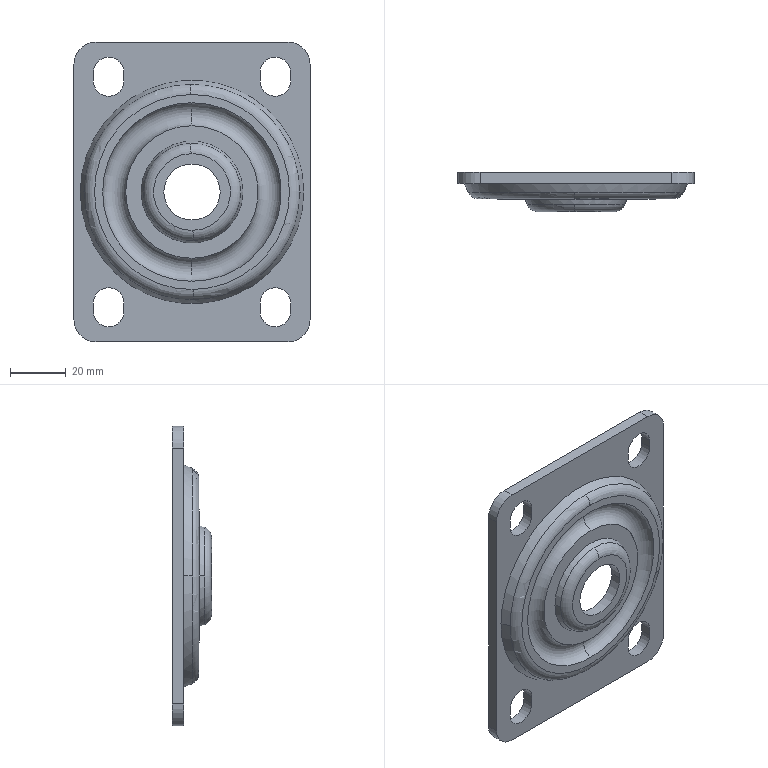Part | NX | features solid 2 | 1 solid | 54 faces | box 85 x 14.1 x 108 mm | volume 38960 mm3 | plane 20 | cylinder 14 | torus 12 | cone 8 | commonest cylinder face diameters 11 x8 16 x4 20.3 x2